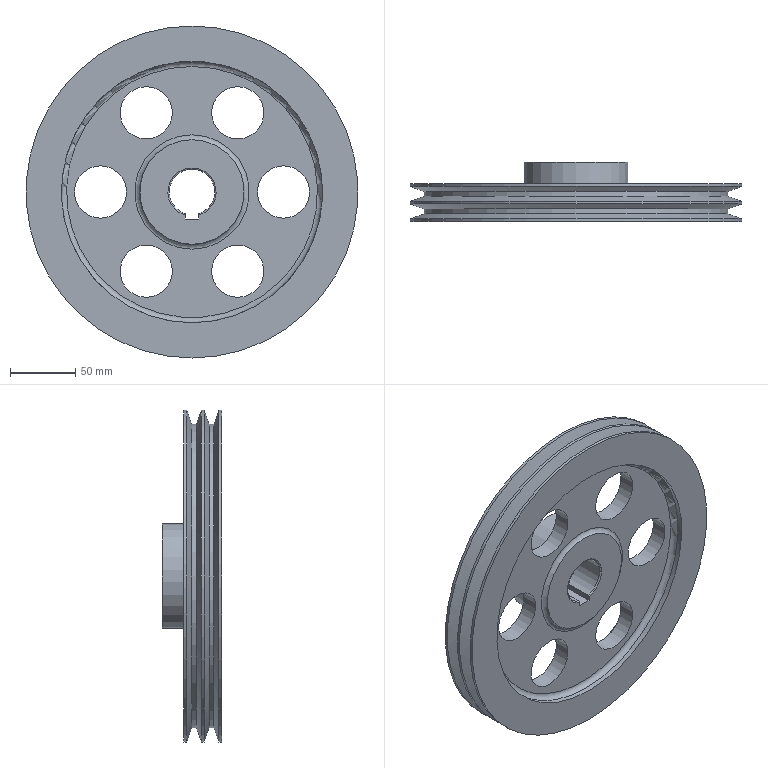Part | NX | features DATUM_CSYS 9, SKETCH 8, EXTRACT_DATUM_AXIS 6, EXTRACT_FACE 6, HOLE PACKAGE 6, SIMPLE HOLE 6, Instance Feature 5, BLEND 2, EXTRUDE 1, Pattern Feature 1, SWP104 1 | 1 solid | 34 faces | box 254 x 45.355 x 254 mm | volume 836856 mm3 | cylinder 15 | plane 9 | torus 6 | cone 4 | commonest cylinder face diameters 40 x6 254 x3 200 x2 232 x2 35 x1 80 x1
STEP:
#1=CARTESIAN_POINT('',(0.,0.,-40.));
#2=VERTEX_POINT('',#1);
#3=CARTESIAN_POINT('',(0.,0.,0.));
#4=DIRECTION('',(0.,-1.,0.));
#5=DIRECTION('',(0.,0.,-1.));
#6=AXIS2_PLACEMENT_3D('',#3,#4,#5);
#7=CIRCLE('',#6,40.);
#8=EDGE_CURVE('',#2,#2,#7,.T.);
#9=ORIENTED_EDGE('',*,*,#8,.T.);
#10=EDGE_LOOP('',(#9));
#11=FACE_BOUND('',#10,.T.);
#12=CARTESIAN_POINT('',(-5.,0.,-17.812));
#13=VERTEX_POINT('',#12);
#14=CARTESIAN_POINT('',(-5.,0.,-20.8));
#15=VERTEX_POINT('',#14);
#16=CARTESIAN_POINT('',(-5.,0.,40.));
#17=DIRECTION('',(0.,0.,-1.));
#18=VECTOR('',#17,1000.);
#19=LINE('',#16,#18);
#20=EDGE_CURVE('',#13,#15,#19,.T.);
#21=ORIENTED_EDGE('',*,*,#20,.F.);
#22=CARTESIAN_POINT('',(5.,0.,-17.812));
#23=VERTEX_POINT('',#22);
#24=CARTESIAN_POINT('',(0.,0.,0.));
#25=DIRECTION('',(0.,1.,0.));
#26=DIRECTION('',(0.,0.,1.));
#27=AXIS2_PLACEMENT_3D('',#24,#25,#26);
#28=CIRCLE('',#27,18.5);
#29=EDGE_CURVE('',#13,#23,#28,.T.);
#30=ORIENTED_EDGE('',*,*,#29,.T.);
#31=CARTESIAN_POINT('',(5.,0.,-20.8));
#32=VERTEX_POINT('',#31);
#33=CARTESIAN_POINT('',(5.,0.,40.));
#34=DIRECTION('',(0.,0.,1.));
#35=VECTOR('',#34,1000.);
#36=LINE('',#33,#35);
#37=EDGE_CURVE('',#32,#23,#36,.T.);
#38=ORIENTED_EDGE('',*,*,#37,.F.);
#39=CARTESIAN_POINT('',(0.,0.,-20.8));
#40=DIRECTION('',(1.,0.,0.));
#41=VECTOR('',#40,1000.);
#42=LINE('',#39,#41);
#43=EDGE_CURVE('',#15,#32,#42,.T.);
#44=ORIENTED_EDGE('',*,*,#43,.F.);
#45=EDGE_LOOP('',(#21,#30,#38,#44));
#46=FACE_BOUND('',#45,.T.);
#47=CARTESIAN_POINT('',(0.,0.,40.));
#48=DIRECTION('',(0.,1.,0.));
#49=DIRECTION('',(0.,0.,1.));
#50=AXIS2_PLACEMENT_3D('',#47,#48,#49);
#51=PLANE('',#50);
#52=ADVANCED_FACE('',(#11,#46),#51,.F.);
#53=CARTESIAN_POINT('',(5.,1.,-16.771));
#54=VERTEX_POINT('',#53);
#55=CARTESIAN_POINT('',(5.,39.,-16.771));
#56=VERTEX_POINT('',#55);
#57=CARTESIAN_POINT('',(5.,0.,-16.771));
#58=DIRECTION('',(0.,-1.,0.));
#59=VECTOR('',#58,1000.);
#60=LINE('',#57,#59);
#61=EDGE_CURVE('',#54,#56,#60,.F.);
#62=ORIENTED_EDGE('',*,*,#61,.F.);
#63=CARTESIAN_POINT('',(-5.,1.,-16.771));
#64=VERTEX_POINT('',#63);
#65=CARTESIAN_POINT('',(0.,1.,0.));
#66=DIRECTION('',(0.,1.,0.));
#67=DIRECTION('',(0.,0.,1.));
#68=AXIS2_PLACEMENT_3D('',#65,#66,#67);
#69=CIRCLE('',#68,17.5);
#70=EDGE_CURVE('',#54,#64,#69,.F.);
#71=ORIENTED_EDGE('',*,*,#70,.T.);
#72=CARTESIAN_POINT('',(-5.,39.,-16.771));
#73=VERTEX_POINT('',#72);
#74=CARTESIAN_POINT('',(-5.,0.,-16.771));
#75=DIRECTION('',(0.,-1.,0.));
#76=VECTOR('',#75,1000.);
#77=LINE('',#74,#76);
#78=EDGE_CURVE('',#73,#64,#77,.T.);
#79=ORIENTED_EDGE('',*,*,#78,.F.);
#80=CARTESIAN_POINT('',(0.,39.,0.));
#81=DIRECTION('',(0.,-1.,0.));
#82=DIRECTION('',(0.,0.,-1.));
#83=AXIS2_PLACEMENT_3D('',#80,#81,#82);
#84=CIRCLE('',#83,17.5);
#85=EDGE_CURVE('',#73,#56,#84,.F.);
#86=ORIENTED_EDGE('',*,*,#85,.T.);
#87=EDGE_LOOP('',(#62,#71,#79,#86));
#88=FACE_BOUND('',#87,.T.);
#89=CARTESIAN_POINT('',(0.,0.,0.));
#90=DIRECTION('',(0.,-1.,0.));
#91=DIRECTION('',(0.,0.,-1.));
#92=AXIS2_PLACEMENT_3D('',#89,#90,#91);
#93=CYLINDRICAL_SURFACE('',#92,17.5);
#94=ADVANCED_FACE('',(#88),#93,.F.);
#95=CARTESIAN_POINT('',(0.,40.,-40.));
#96=VERTEX_POINT('',#95);
#97=CARTESIAN_POINT('',(0.,40.,0.));
#98=DIRECTION('',(0.,-1.,0.));
#99=DIRECTION('',(0.,0.,-1.));
#100=AXIS2_PLACEMENT_3D('',#97,#98,#99);
#101=CIRCLE('',#100,40.);
#102=EDGE_CURVE('',#96,#96,#101,.T.);
#103=ORIENTED_EDGE('',*,*,#102,.F.);
#104=EDGE_LOOP('',(#103));
#105=FACE_BOUND('',#104,.T.);
#106=CARTESIAN_POINT('',(5.,40.,-17.812));
#107=VERTEX_POINT('',#106);
#108=CARTESIAN_POINT('',(5.,40.,-20.8));
#109=VERTEX_POINT('',#108);
#110=CARTESIAN_POINT('',(5.,40.,17.5));
#111=DIRECTION('',(0.,0.,-1.));
#112=VECTOR('',#111,1000.);
#113=LINE('',#110,#112);
#114=EDGE_CURVE('',#107,#109,#113,.T.);
#115=ORIENTED_EDGE('',*,*,#114,.F.);
#116=CARTESIAN_POINT('',(-5.,40.,-17.812));
#117=VERTEX_POINT('',#116);
#118=CARTESIAN_POINT('',(0.,40.,0.));
#119=DIRECTION('',(0.,-1.,0.));
#120=DIRECTION('',(0.,0.,-1.));
#121=AXIS2_PLACEMENT_3D('',#118,#119,#120);
#122=CIRCLE('',#121,18.5);
#123=EDGE_CURVE('',#107,#117,#122,.T.);
#124=ORIENTED_EDGE('',*,*,#123,.T.);
#125=CARTESIAN_POINT('',(-5.,40.,-20.8));
#126=VERTEX_POINT('',#125);
#127=CARTESIAN_POINT('',(-5.,40.,17.5));
#128=DIRECTION('',(0.,0.,1.));
#129=VECTOR('',#128,1000.);
#130=LINE('',#127,#129);
#131=EDGE_CURVE('',#126,#117,#130,.T.);
#132=ORIENTED_EDGE('',*,*,#131,.F.);
#133=CARTESIAN_POINT('',(0.,40.,-20.8));
#134=DIRECTION('',(-1.,0.,0.));
#135=VECTOR('',#134,1000.);
#136=LINE('',#133,#135);
#137=EDGE_CURVE('',#109,#126,#136,.T.);
#138=ORIENTED_EDGE('',*,*,#137,.F.);
#139=EDGE_LOOP('',(#115,#124,#132,#138));
#140=FACE_BOUND('',#139,.T.);
#141=CARTESIAN_POINT('',(0.,40.,17.5));
#142=DIRECTION('',(0.,-1.,0.));
#143=DIRECTION('',(0.,0.,-1.));
#144=AXIS2_PLACEMENT_3D('',#141,#142,#143);
#145=PLANE('',#144);
#146=ADVANCED_FACE('',(#105,#140),#145,.F.);
#147=CARTESIAN_POINT('',(0.,-5.355,-100.));
#148=VERTEX_POINT('',#147);
#149=CARTESIAN_POINT('',(0.,-5.355,0.));
#150=DIRECTION('',(0.,-1.,0.));
#151=DIRECTION('',(0.,0.,-1.));
#152=AXIS2_PLACEMENT_3D('',#149,#150,#151);
#153=CIRCLE('',#152,100.);
#154=EDGE_CURVE('',#148,#148,#153,.T.);
#155=ORIENTED_EDGE('',*,*,#154,.F.);
#156=EDGE_LOOP('',(#155));
#157=FACE_BOUND('',#156,.T.);
#158=CARTESIAN_POINT('',(0.,-5.355,-127.));
#159=VERTEX_POINT('',#158);
#160=CARTESIAN_POINT('',(0.,-5.355,0.));
#161=DIRECTION('',(0.,-1.,0.));
#162=DIRECTION('',(0.,0.,-1.));
#163=AXIS2_PLACEMENT_3D('',#160,#161,#162);
#164=CIRCLE('',#163,127.);
#165=EDGE_CURVE('',#159,#159,#164,.T.);
#166=ORIENTED_EDGE('',*,*,#165,.T.);
#167=EDGE_LOOP('',(#166));
#168=FACE_BOUND('',#167,.T.);
#169=CARTESIAN_POINT('',(0.,-5.355,127.));
#170=DIRECTION('',(0.,1.,0.));
#171=DIRECTION('',(0.,0.,1.));
#172=AXIS2_PLACEMENT_3D('',#169,#170,#171);
#173=PLANE('',#172);
#174=ADVANCED_FACE('',(#157,#168),#173,.F.);
#175=CARTESIAN_POINT('',(0.,-1.294,100.));
#176=VERTEX_POINT('',#175);
#177=CARTESIAN_POINT('',(0.,-1.294,0.));
#178=DIRECTION('',(0.,1.,0.));
#179=DIRECTION('',(0.,0.,1.));
#180=AXIS2_PLACEMENT_3D('',#177,#178,#179);
#181=CIRCLE('',#180,100.);
#182=EDGE_CURVE('',#176,#176,#181,.T.);
#183=ORIENTED_EDGE('',*,*,#182,.T.);
#184=EDGE_LOOP('',(#183));
#185=FACE_BOUND('',#184,.T.);
#186=ORIENTED_EDGE('',*,*,#154,.T.);
#187=EDGE_LOOP('',(#186));
#188=FACE_BOUND('',#187,.T.);
#189=CARTESIAN_POINT('',(0.,0.,0.));
#190=DIRECTION('',(0.,-1.,0.));
#191=DIRECTION('',(0.,0.,-1.));
#192=AXIS2_PLACEMENT_3D('',#189,#190,#191);
#193=CYLINDRICAL_SURFACE('',#192,100.);
#194=ADVANCED_FACE('',(#185,#188),#193,.F.);
#195=CARTESIAN_POINT('',(0.,2.706,96.));
#196=VERTEX_POINT('',#195);
#197=CARTESIAN_POINT('',(0.,2.706,0.));
#198=DIRECTION('',(0.,1.,0.));
#199=DIRECTION('',(0.,0.,1.));
#200=AXIS2_PLACEMENT_3D('',#197,#198,#199);
#201=CIRCLE('',#200,96.);
#202=EDGE_CURVE('',#196,#196,#201,.F.);
#203=ORIENTED_EDGE('',*,*,#202,.T.);
#204=EDGE_LOOP('',(#203));
#205=FACE_BOUND('',#204,.T.);
#206=CARTESIAN_POINT('',(-35.,2.706,80.622));
#207=VERTEX_POINT('',#206);
#208=CARTESIAN_POINT('',(-35.,2.706,60.622));
#209=DIRECTION('',(0.,1.,0.));
#210=DIRECTION('',(0.,0.,1.));
#211=AXIS2_PLACEMENT_3D('',#208,#209,#210);
#212=CIRCLE('',#211,20.);
#213=EDGE_CURVE('',#207,#207,#212,.T.);
#214=ORIENTED_EDGE('',*,*,#213,.T.);
#215=EDGE_LOOP('',(#214));
#216=FACE_BOUND('',#215,.T.);
#217=CARTESIAN_POINT('',(35.,2.706,80.622));
#218=VERTEX_POINT('',#217);
#219=CARTESIAN_POINT('',(35.,2.706,60.622));
#220=DIRECTION('',(0.,1.,0.));
#221=DIRECTION('',(0.,0.,1.));
#222=AXIS2_PLACEMENT_3D('',#219,#220,#221);
#223=CIRCLE('',#222,20.);
#224=EDGE_CURVE('',#218,#218,#223,.T.);
#225=ORIENTED_EDGE('',*,*,#224,.T.);
#226=EDGE_LOOP('',(#225));
#227=FACE_BOUND('',#226,.T.);
#228=CARTESIAN_POINT('',(70.,2.706,20.));
#229=VERTEX_POINT('',#228);
#230=CARTESIAN_POINT('',(70.,2.706,0.));
#231=DIRECTION('',(0.,1.,0.));
#232=DIRECTION('',(0.,0.,1.));
#233=AXIS2_PLACEMENT_3D('',#230,#231,#232);
#234=CIRCLE('',#233,20.);
#235=EDGE_CURVE('',#229,#229,#234,.T.);
#236=ORIENTED_EDGE('',*,*,#235,.T.);
#237=EDGE_LOOP('',(#236));
#238=FACE_BOUND('',#237,.T.);
#239=CARTESIAN_POINT('',(35.,2.706,-40.622));
#240=VERTEX_POINT('',#239);
#241=CARTESIAN_POINT('',(35.,2.706,-60.622));
#242=DIRECTION('',(0.,1.,0.));
#243=DIRECTION('',(0.,0.,1.));
#244=AXIS2_PLACEMENT_3D('',#241,#242,#243);
#245=CIRCLE('',#244,20.);
#246=EDGE_CURVE('',#240,#240,#245,.T.);
#247=ORIENTED_EDGE('',*,*,#246,.T.);
#248=EDGE_LOOP('',(#247));
#249=FACE_BOUND('',#248,.T.);
#250=CARTESIAN_POINT('',(-35.,2.706,-40.622));
#251=VERTEX_POINT('',#250);
#252=CARTESIAN_POINT('',(-35.,2.706,-60.622));
#253=DIRECTION('',(0.,1.,0.));
#254=DIRECTION('',(0.,0.,1.));
#255=AXIS2_PLACEMENT_3D('',#252,#253,#254);
#256=CIRCLE('',#255,20.);
#257=EDGE_CURVE('',#251,#251,#256,.T.);
#258=ORIENTED_EDGE('',*,*,#257,.T.);
#259=EDGE_LOOP('',(#258));
#260=FACE_BOUND('',#259,.T.);
#261=CARTESIAN_POINT('',(-70.,2.706,20.));
#262=VERTEX_POINT('',#261);
#263=CARTESIAN_POINT('',(-70.,2.706,0.));
#264=DIRECTION('',(0.,1.,0.));
#265=DIRECTION('',(0.,0.,1.));
#266=AXIS2_PLACEMENT_3D('',#263,#264,#265);
#267=CIRCLE('',#266,20.);
#268=EDGE_CURVE('',#262,#262,#267,.T.);
#269=ORIENTED_EDGE('',*,*,#268,.T.);
#270=EDGE_LOOP('',(#269));
#271=FACE_BOUND('',#270,.T.);
#272=CARTESIAN_POINT('',(0.,2.706,-43.785));
#273=VERTEX_POINT('',#272);
#274=CARTESIAN_POINT('',(0.,2.706,0.));
#275=DIRECTION('',(0.,-1.,0.));
#276=DIRECTION('',(0.,0.,-1.));
#277=AXIS2_PLACEMENT_3D('',#274,#275,#276);
#278=CIRCLE('',#277,43.785);
#279=EDGE_CURVE('',#273,#273,#278,.T.);
#280=ORIENTED_EDGE('',*,*,#279,.F.);
#281=EDGE_LOOP('',(#280));
#282=FACE_BOUND('',#281,.T.);
#283=CARTESIAN_POINT('',(0.,2.706,100.));
#284=DIRECTION('',(0.,1.,0.));
#285=DIRECTION('',(0.,0.,1.));
#286=AXIS2_PLACEMENT_3D('',#283,#284,#285);
#287=PLANE('',#286);
#288=ADVANCED_FACE('',(#205,#216,#227,#238,#249,#260,#271,#282),#287,.F.);
#289=ORIENTED_EDGE('',*,*,#8,.F.);
#290=EDGE_LOOP('',(#289));
#291=FACE_BOUND('',#290,.T.);
#292=ORIENTED_EDGE('',*,*,#279,.T.);
#293=EDGE_LOOP('',(#292));
#294=FACE_BOUND('',#293,.T.);
#295=CARTESIAN_POINT('',(0.,-1.294,0.));
#296=DIRECTION('',(0.,-1.,0.));
#297=DIRECTION('',(0.,0.,-1.));
#298=AXIS2_PLACEMENT_3D('',#295,#296,#297);
#299=TOROIDAL_SURFACE('',#298,43.785,4.);
#300=ADVANCED_FACE('',(#291,#294),#299,.F.);
#301=CARTESIAN_POINT('',(0.,19.495,-40.));
#302=VERTEX_POINT('',#301);
#303=CARTESIAN_POINT('',(0.,19.495,0.));
#304=DIRECTION('',(0.,-1.,0.));
#305=DIRECTION('',(0.,0.,-1.));
#306=AXIS2_PLACEMENT_3D('',#303,#304,#305);
#307=CIRCLE('',#306,40.);
#308=EDGE_CURVE('',#302,#302,#307,.F.);
#309=ORIENTED_EDGE('',*,*,#308,.T.);
#310=EDGE_LOOP('',(#309));
#311=FACE_BOUND('',#310,.T.);
#312=ORIENTED_EDGE('',*,*,#102,.T.);
#313=EDGE_LOOP('',(#312));
#314=FACE_BOUND('',#313,.T.);
#315=CARTESIAN_POINT('',(0.,0.,0.));
#316=DIRECTION('',(0.,-1.,0.));
#317=DIRECTION('',(0.,0.,-1.));
#318=AXIS2_PLACEMENT_3D('',#315,#316,#317);
#319=CYLINDRICAL_SURFACE('',#318,40.);
#320=ADVANCED_FACE('',(#311,#314),#319,.T.);
#321=CARTESIAN_POINT('',(0.,15.495,-44.));
#322=VERTEX_POINT('',#321);
#323=CARTESIAN_POINT('',(0.,15.495,0.));
#324=DIRECTION('',(0.,-1.,0.));
#325=DIRECTION('',(0.,0.,-1.));
#326=AXIS2_PLACEMENT_3D('',#323,#324,#325);
#327=CIRCLE('',#326,44.);
#328=EDGE_CURVE('',#322,#322,#327,.T.);
#329=ORIENTED_EDGE('',*,*,#328,.T.);
#330=EDGE_LOOP('',(#329));
#331=FACE_BOUND('',#330,.T.);
#332=CARTESIAN_POINT('',(0.,15.495,-96.));
#333=VERTEX_POINT('',#332);
#334=CARTESIAN_POINT('',(0.,15.495,0.));
#335=DIRECTION('',(0.,-1.,0.));
#336=DIRECTION('',(0.,0.,-1.));
#337=AXIS2_PLACEMENT_3D('',#334,#335,#336);
#338=CIRCLE('',#337,96.);
#339=EDGE_CURVE('',#333,#333,#338,.F.);
#340=ORIENTED_EDGE('',*,*,#339,.T.);
#341=EDGE_LOOP('',(#340));
#342=FACE_BOUND('',#341,.T.);
#343=CARTESIAN_POINT('',(-35.,15.495,40.622));
#344=VERTEX_POINT('',#343);
#345=CARTESIAN_POINT('',(-35.,15.495,60.622));
#346=DIRECTION('',(0.,-1.,0.));
#347=DIRECTION('',(0.,0.,-1.));
#348=AXIS2_PLACEMENT_3D('',#345,#346,#347);
#349=CIRCLE('',#348,20.);
#350=EDGE_CURVE('',#344,#344,#349,.T.);
#351=ORIENTED_EDGE('',*,*,#350,.T.);
#352=EDGE_LOOP('',(#351));
#353=FACE_BOUND('',#352,.T.);
#354=CARTESIAN_POINT('',(35.,15.495,40.622));
#355=VERTEX_POINT('',#354);
#356=CARTESIAN_POINT('',(35.,15.495,60.622));
#357=DIRECTION('',(0.,-1.,0.));
#358=DIRECTION('',(0.,0.,-1.));
#359=AXIS2_PLACEMENT_3D('',#356,#357,#358);
#360=CIRCLE('',#359,20.);
#361=EDGE_CURVE('',#355,#355,#360,.T.);
#362=ORIENTED_EDGE('',*,*,#361,.T.);
#363=EDGE_LOOP('',(#362));
#364=FACE_BOUND('',#363,.T.);
#365=CARTESIAN_POINT('',(70.,15.495,-20.));
#366=VERTEX_POINT('',#365);
#367=CARTESIAN_POINT('',(70.,15.495,0.));
#368=DIRECTION('',(0.,-1.,0.));
#369=DIRECTION('',(0.,0.,-1.));
#370=AXIS2_PLACEMENT_3D('',#367,#368,#369);
#371=CIRCLE('',#370,20.);
#372=EDGE_CURVE('',#366,#366,#371,.T.);
#373=ORIENTED_EDGE('',*,*,#372,.T.);
#374=EDGE_LOOP('',(#373));
#375=FACE_BOUND('',#374,.T.);
#376=CARTESIAN_POINT('',(35.,15.495,-80.622));
#377=VERTEX_POINT('',#376);
#378=CARTESIAN_POINT('',(35.,15.495,-60.622));
#379=DIRECTION('',(0.,-1.,0.));
#380=DIRECTION('',(0.,0.,-1.));
#381=AXIS2_PLACEMENT_3D('',#378,#379,#380);
#382=CIRCLE('',#381,20.);
#383=EDGE_CURVE('',#377,#377,#382,.T.);
#384=ORIENTED_EDGE('',*,*,#383,.T.);
#385=EDGE_LOOP('',(#384));
#386=FACE_BOUND('',#385,.T.);
#387=CARTESIAN_POINT('',(-35.,15.495,-80.622));
#388=VERTEX_POINT('',#387);
#389=CARTESIAN_POINT('',(-35.,15.495,-60.622));
#390=DIRECTION('',(0.,-1.,0.));
#391=DIRECTION('',(0.,0.,-1.));
#392=AXIS2_PLACEMENT_3D('',#389,#390,#391);
#393=CIRCLE('',#392,20.);
#394=EDGE_CURVE('',#388,#388,#393,.T.);
#395=ORIENTED_EDGE('',*,*,#394,.T.);
#396=EDGE_LOOP('',(#395));
#397=FACE_BOUND('',#396,.T.);
#398=CARTESIAN_POINT('',(-70.,15.495,-20.));
#399=VERTEX_POINT('',#398);
#400=CARTESIAN_POINT('',(-70.,15.495,0.));
#401=DIRECTION('',(0.,-1.,0.));
#402=DIRECTION('',(0.,0.,-1.));
#403=AXIS2_PLACEMENT_3D('',#400,#401,#402);
#404=CIRCLE('',#403,20.);
#405=EDGE_CURVE('',#399,#399,#404,.T.);
#406=ORIENTED_EDGE('',*,*,#405,.T.);
#407=EDGE_LOOP('',(#406));
#408=FACE_BOUND('',#407,.T.);
#409=CARTESIAN_POINT('',(0.,15.495,40.));
#410=DIRECTION('',(0.,-1.,0.));
#411=DIRECTION('',(0.,0.,-1.));
#412=AXIS2_PLACEMENT_3D('',#409,#410,#411);
#413=PLANE('',#412);
#414=ADVANCED_FACE('',(#331,#342,#353,#364,#375,#386,#397,#408),#413,.F.);
#415=CARTESIAN_POINT('',(0.,19.495,-100.));
#416=VERTEX_POINT('',#415);
#417=CARTESIAN_POINT('',(0.,19.495,0.));
#418=DIRECTION('',(0.,-1.,0.));
#419=DIRECTION('',(0.,0.,-1.));
#420=AXIS2_PLACEMENT_3D('',#417,#418,#419);
#421=CIRCLE('',#420,100.);
#422=EDGE_CURVE('',#416,#416,#421,.T.);
#423=ORIENTED_EDGE('',*,*,#422,.T.);
#424=EDGE_LOOP('',(#423));
#425=FACE_BOUND('',#424,.T.);
#426=CARTESIAN_POINT('',(0.,23.495,-100.));
#427=VERTEX_POINT('',#426);
#428=CARTESIAN_POINT('',(0.,23.495,0.));
#429=DIRECTION('',(0.,-1.,0.));
#430=DIRECTION('',(0.,0.,-1.));
#431=AXIS2_PLACEMENT_3D('',#428,#429,#430);
#432=CIRCLE('',#431,100.);
#433=EDGE_CURVE('',#427,#427,#432,.T.);
#434=ORIENTED_EDGE('',*,*,#433,.F.);
#435=EDGE_LOOP('',(#434));
#436=FACE_BOUND('',#435,.T.);
#437=CARTESIAN_POINT('',(0.,0.,0.));
#438=DIRECTION('',(0.,-1.,0.));
#439=DIRECTION('',(0.,0.,-1.));
#440=AXIS2_PLACEMENT_3D('',#437,#438,#439);
#441=CYLINDRICAL_SURFACE('',#440,100.);
#442=ADVANCED_FACE('',(#425,#436),#441,.F.);
#443=CARTESIAN_POINT('',(0.,23.495,-127.));
#444=VERTEX_POINT('',#443);
#445=CARTESIAN_POINT('',(0.,23.495,0.));
#446=DIRECTION('',(0.,-1.,0.));
#447=DIRECTION('',(0.,0.,-1.));
#448=AXIS2_PLACEMENT_3D('',#445,#446,#447);
#449=CIRCLE('',#448,127.);
#450=EDGE_CURVE('',#444,#444,#449,.T.);
#451=ORIENTED_EDGE('',*,*,#450,.F.);
#452=EDGE_LOOP('',(#451));
#453=FACE_BOUND('',#452,.T.);
#454=ORIENTED_EDGE('',*,*,#433,.T.);
#455=EDGE_LOOP('',(#454));
#456=FACE_BOUND('',#455,.T.);
#457=CARTESIAN_POINT('',(0.,23.495,100.));
#458=DIRECTION('',(0.,-1.,0.));
#459=DIRECTION('',(0.,0.,-1.));
#460=AXIS2_PLACEMENT_3D('',#457,#458,#459);
#461=PLANE('',#460);
#462=ADVANCED_FACE('',(#453,#456),#461,.F.);
#463=CARTESIAN_POINT('',(0.,21.395,-127.));
#464=VERTEX_POINT('',#463);
#465=CARTESIAN_POINT('',(0.,21.395,0.));
#466=DIRECTION('',(0.,-1.,0.));
#467=DIRECTION('',(0.,0.,-1.));
#468=AXIS2_PLACEMENT_3D('',#465,#466,#467);
#469=CIRCLE('',#468,127.);
#470=EDGE_CURVE('',#464,#464,#469,.T.);
#471=ORIENTED_EDGE('',*,*,#470,.F.);
#472=EDGE_LOOP('',(#471));
#473=FACE_BOUND('',#472,.T.);
#474=ORIENTED_EDGE('',*,*,#450,.T.);
#475=EDGE_LOOP('',(#474));
#476=FACE_BOUND('',#475,.T.);
#477=CARTESIAN_POINT('',(0.,0.,0.));
#478=DIRECTION('',(0.,-1.,0.));
#479=DIRECTION('',(0.,0.,-1.));
#480=AXIS2_PLACEMENT_3D('',#477,#478,#479);
#481=CYLINDRICAL_SURFACE('',#480,127.);
#482=ADVANCED_FACE('',(#473,#476),#481,.T.);
#483=CARTESIAN_POINT('',(0.,17.608,-116.));
#484=VERTEX_POINT('',#483);
#485=CARTESIAN_POINT('',(0.,17.608,0.));
#486=DIRECTION('',(0.,-1.,0.));
#487=DIRECTION('',(0.,0.,-1.));
#488=AXIS2_PLACEMENT_3D('',#485,#486,#487);
#489=CIRCLE('',#488,116.);
#490=EDGE_CURVE('',#484,#484,#489,.T.);
#491=ORIENTED_EDGE('',*,*,#490,.F.);
#492=EDGE_LOOP('',(#491));
#493=FACE_BOUND('',#492,.T.);
#494=ORIENTED_EDGE('',*,*,#470,.T.);
#495=EDGE_LOOP('',(#494));
#496=FACE_BOUND('',#495,.T.);
#497=CARTESIAN_POINT('',(0.,21.395,0.));
#498=DIRECTION('',(0.,1.,0.));
#499=DIRECTION('',(0.,0.,1.));
#500=AXIS2_PLACEMENT_3D('',#497,#498,#499);
#501=CONICAL_SURFACE('',#500,127.,1.239);
#502=ADVANCED_FACE('',(#493,#496),#501,.T.);
#503=CARTESIAN_POINT('',(0.,13.908,-116.));
#504=VERTEX_POINT('',#503);
#505=CARTESIAN_POINT('',(0.,13.908,0.));
#506=DIRECTION('',(0.,-1.,0.));
#507=DIRECTION('',(0.,0.,-1.));
#508=AXIS2_PLACEMENT_3D('',#505,#506,#507);
#509=CIRCLE('',#508,116.);
#510=EDGE_CURVE('',#504,#504,#509,.T.);
#511=ORIENTED_EDGE('',*,*,#510,.F.);
#512=EDGE_LOOP('',(#511));
#513=FACE_BOUND('',#512,.T.);
#514=ORIENTED_EDGE('',*,*,#490,.T.);
#515=EDGE_LOOP('',(#514));
#516=FACE_BOUND('',#515,.T.);
#517=CARTESIAN_POINT('',(0.,0.,0.));
#518=DIRECTION('',(0.,-1.,0.));
#519=DIRECTION('',(0.,0.,-1.));
#520=AXIS2_PLACEMENT_3D('',#517,#518,#519);
#521=CYLINDRICAL_SURFACE('',#520,116.);
#522=ADVANCED_FACE('',(#513,#516),#521,.T.);
#523=CARTESIAN_POINT('',(0.,10.12,-127.));
#524=VERTEX_POINT('',#523);
#525=CARTESIAN_POINT('',(0.,10.12,0.));
#526=DIRECTION('',(0.,-1.,0.));
#527=DIRECTION('',(0.,0.,-1.));
#528=AXIS2_PLACEMENT_3D('',#525,#526,#527);
#529=CIRCLE('',#528,127.);
#530=EDGE_CURVE('',#524,#524,#529,.T.);
#531=ORIENTED_EDGE('',*,*,#530,.F.);
#532=EDGE_LOOP('',(#531));
#533=FACE_BOUND('',#532,.T.);
#534=ORIENTED_EDGE('',*,*,#510,.T.);
#535=EDGE_LOOP('',(#534));
#536=FACE_BOUND('',#535,.T.);
#537=CARTESIAN_POINT('',(0.,13.908,0.));
#538=DIRECTION('',(0.,-1.,0.));
#539=DIRECTION('',(0.,0.,-1.));
#540=AXIS2_PLACEMENT_3D('',#537,#538,#539);
#541=CONICAL_SURFACE('',#540,116.,1.239);
#542=ADVANCED_FACE('',(#533,#536),#541,.T.);
#543=CARTESIAN_POINT('',(0.,8.02,-127.));
#544=VERTEX_POINT('',#543);
#545=CARTESIAN_POINT('',(0.,8.02,0.));
#546=DIRECTION('',(0.,-1.,0.));
#547=DIRECTION('',(0.,0.,-1.));
#548=AXIS2_PLACEMENT_3D('',#545,#546,#547);
#549=CIRCLE('',#548,127.);
#550=EDGE_CURVE('',#544,#544,#549,.T.);
#551=ORIENTED_EDGE('',*,*,#550,.F.);
#552=EDGE_LOOP('',(#551));
#553=FACE_BOUND('',#552,.T.);
#554=ORIENTED_EDGE('',*,*,#530,.T.);
#555=EDGE_LOOP('',(#554));
#556=FACE_BOUND('',#555,.T.);
#557=CARTESIAN_POINT('',(0.,0.,0.));
#558=DIRECTION('',(0.,-1.,0.));
#559=DIRECTION('',(0.,0.,-1.));
#560=AXIS2_PLACEMENT_3D('',#557,#558,#559);
#561=CYLINDRICAL_SURFACE('',#560,127.);
#562=ADVANCED_FACE('',(#553,#556),#561,.T.);
#563=CARTESIAN_POINT('',(0.,4.233,-116.));
#564=VERTEX_POINT('',#563);
#565=CARTESIAN_POINT('',(0.,4.233,0.));
#566=DIRECTION('',(0.,-1.,0.));
#567=DIRECTION('',(0.,0.,-1.));
#568=AXIS2_PLACEMENT_3D('',#565,#566,#567);
#569=CIRCLE('',#568,116.);
#570=EDGE_CURVE('',#564,#564,#569,.T.);
#571=ORIENTED_EDGE('',*,*,#570,.F.);
#572=EDGE_LOOP('',(#571));
#573=FACE_BOUND('',#572,.T.);
#574=ORIENTED_EDGE('',*,*,#550,.T.);
#575=EDGE_LOOP('',(#574));
#576=FACE_BOUND('',#575,.T.);
#577=CARTESIAN_POINT('',(0.,8.02,0.));
#578=DIRECTION('',(0.,1.,0.));
#579=DIRECTION('',(0.,0.,1.));
#580=AXIS2_PLACEMENT_3D('',#577,#578,#579);
#581=CONICAL_SURFACE('',#580,127.,1.239);
#582=ADVANCED_FACE('',(#573,#576),#581,.T.);
#583=CARTESIAN_POINT('',(0.,0.5326,-116.));
#584=VERTEX_POINT('',#583);
#585=CARTESIAN_POINT('',(0.,0.5326,0.));
#586=DIRECTION('',(0.,-1.,0.));
#587=DIRECTION('',(0.,0.,-1.));
#588=AXIS2_PLACEMENT_3D('',#585,#586,#587);
#589=CIRCLE('',#588,116.);
#590=EDGE_CURVE('',#584,#584,#589,.T.);
#591=ORIENTED_EDGE('',*,*,#590,.F.);
#592=EDGE_LOOP('',(#591));
#593=FACE_BOUND('',#592,.T.);
#594=ORIENTED_EDGE('',*,*,#570,.T.);
#595=EDGE_LOOP('',(#594));
#596=FACE_BOUND('',#595,.T.);
#597=CARTESIAN_POINT('',(0.,0.,0.));
#598=DIRECTION('',(0.,-1.,0.));
#599=DIRECTION('',(0.,0.,-1.));
#600=AXIS2_PLACEMENT_3D('',#597,#598,#599);
#601=CYLINDRICAL_SURFACE('',#600,116.);
#602=ADVANCED_FACE('',(#593,#596),#601,.T.);
#603=CARTESIAN_POINT('',(0.,-3.255,-127.));
#604=VERTEX_POINT('',#603);
#605=CARTESIAN_POINT('',(0.,-3.255,0.));
#606=DIRECTION('',(0.,-1.,0.));
#607=DIRECTION('',(0.,0.,-1.));
#608=AXIS2_PLACEMENT_3D('',#605,#606,#607);
#609=CIRCLE('',#608,127.);
#610=EDGE_CURVE('',#604,#604,#609,.T.);
#611=ORIENTED_EDGE('',*,*,#610,.F.);
#612=EDGE_LOOP('',(#611));
#613=FACE_BOUND('',#612,.T.);
#614=ORIENTED_EDGE('',*,*,#590,.T.);
#615=EDGE_LOOP('',(#614));
#616=FACE_BOUND('',#615,.T.);
#617=CARTESIAN_POINT('',(0.,0.5326,0.));
#618=DIRECTION('',(0.,-1.,0.));
#619=DIRECTION('',(0.,0.,-1.));
#620=AXIS2_PLACEMENT_3D('',#617,#618,#619);
#621=CONICAL_SURFACE('',#620,116.,1.239);
#622=ADVANCED_FACE('',(#613,#616),#621,.T.);
#623=ORIENTED_EDGE('',*,*,#165,.F.);
#624=EDGE_LOOP('',(#623));
#625=FACE_BOUND('',#624,.T.);
#626=ORIENTED_EDGE('',*,*,#610,.T.);
#627=EDGE_LOOP('',(#626));
#628=FACE_BOUND('',#627,.T.);
#629=CARTESIAN_POINT('',(0.,0.,0.));
#630=DIRECTION('',(0.,-1.,0.));
#631=DIRECTION('',(0.,0.,-1.));
#632=AXIS2_PLACEMENT_3D('',#629,#630,#631);
#633=CYLINDRICAL_SURFACE('',#632,127.);
#634=ADVANCED_FACE('',(#625,#628),#633,.T.);
#635=ORIENTED_EDGE('',*,*,#405,.F.);
#636=EDGE_LOOP('',(#635));
#637=FACE_BOUND('',#636,.T.);
#638=ORIENTED_EDGE('',*,*,#268,.F.);
#639=EDGE_LOOP('',(#638));
#640=FACE_BOUND('',#639,.T.);
#641=CARTESIAN_POINT('',(-70.,15.495,0.));
#642=DIRECTION('',(0.,-1.,0.));
#643=DIRECTION('',(0.,0.,-1.));
#644=AXIS2_PLACEMENT_3D('',#641,#642,#643);
#645=CYLINDRICAL_SURFACE('',#644,20.);
#646=ADVANCED_FACE('',(#637,#640),#645,.F.);
#647=ORIENTED_EDGE('',*,*,#394,.F.);
#648=EDGE_LOOP('',(#647));
#649=FACE_BOUND('',#648,.T.);
#650=ORIENTED_EDGE('',*,*,#257,.F.);
#651=EDGE_LOOP('',(#650));
#652=FACE_BOUND('',#651,.T.);
#653=CARTESIAN_POINT('',(-35.,15.495,-60.622));
#654=DIRECTION('',(0.,-1.,0.));
#655=DIRECTION('',(0.,0.,-1.));
#656=AXIS2_PLACEMENT_3D('',#653,#654,#655);
#657=CYLINDRICAL_SURFACE('',#656,20.);
#658=ADVANCED_FACE('',(#649,#652),#657,.F.);
#659=ORIENTED_EDGE('',*,*,#383,.F.);
#660=EDGE_LOOP('',(#659));
#661=FACE_BOUND('',#660,.T.);
#662=ORIENTED_EDGE('',*,*,#246,.F.);
#663=EDGE_LOOP('',(#662));
#664=FACE_BOUND('',#663,.T.);
#665=CARTESIAN_POINT('',(35.,15.495,-60.622));
#666=DIRECTION('',(0.,-1.,0.));
#667=DIRECTION('',(0.,0.,-1.));
#668=AXIS2_PLACEMENT_3D('',#665,#666,#667);
#669=CYLINDRICAL_SURFACE('',#668,20.);
#670=ADVANCED_FACE('',(#661,#664),#669,.F.);
#671=ORIENTED_EDGE('',*,*,#372,.F.);
#672=EDGE_LOOP('',(#671));
#673=FACE_BOUND('',#672,.T.);
#674=ORIENTED_EDGE('',*,*,#235,.F.);
#675=EDGE_LOOP('',(#674));
#676=FACE_BOUND('',#675,.T.);
#677=CARTESIAN_POINT('',(70.,15.495,0.));
#678=DIRECTION('',(0.,-1.,0.));
#679=DIRECTION('',(0.,0.,-1.));
#680=AXIS2_PLACEMENT_3D('',#677,#678,#679);
#681=CYLINDRICAL_SURFACE('',#680,20.);
#682=ADVANCED_FACE('',(#673,#676),#681,.F.);
#683=ORIENTED_EDGE('',*,*,#361,.F.);
#684=EDGE_LOOP('',(#683));
#685=FACE_BOUND('',#684,.T.);
#686=ORIENTED_EDGE('',*,*,#224,.F.);
#687=EDGE_LOOP('',(#686));
#688=FACE_BOUND('',#687,.T.);
#689=CARTESIAN_POINT('',(35.,15.495,60.622));
#690=DIRECTION('',(0.,-1.,0.));
#691=DIRECTION('',(0.,0.,-1.));
#692=AXIS2_PLACEMENT_3D('',#689,#690,#691);
#693=CYLINDRICAL_SURFACE('',#692,20.);
#694=ADVANCED_FACE('',(#685,#688),#693,.F.);
#695=ORIENTED_EDGE('',*,*,#350,.F.);
#696=EDGE_LOOP('',(#695));
#697=FACE_BOUND('',#696,.T.);
#698=ORIENTED_EDGE('',*,*,#213,.F.);
#699=EDGE_LOOP('',(#698));
#700=FACE_BOUND('',#699,.T.);
#701=CARTESIAN_POINT('',(-35.,15.495,60.622));
#702=DIRECTION('',(0.,-1.,0.));
#703=DIRECTION('',(0.,0.,-1.));
#704=AXIS2_PLACEMENT_3D('',#701,#702,#703);
#705=CYLINDRICAL_SURFACE('',#704,20.);
#706=ADVANCED_FACE('',(#697,#700),#705,.F.);
#707=ORIENTED_EDGE('',*,*,#78,.T.);
#708=CARTESIAN_POINT('',(-5.,1.,-16.771));
#709=CARTESIAN_POINT('',(-5.,0.4608,-16.771));
#710=CARTESIAN_POINT('',(-5.,0.,-17.273));
#711=CARTESIAN_POINT('',(-5.,0.,-17.812));
#712=B_SPLINE_CURVE_WITH_KNOTS('',3,(#708,#709,#710,#711),.UNSPECIFIED.,.F.,.F.,(4,4),(0.,0.001594),.UNSPECIFIED.);
#713=EDGE_CURVE('',#64,#13,#712,.T.);
#714=ORIENTED_EDGE('',*,*,#713,.T.);
#715=ORIENTED_EDGE('',*,*,#20,.T.);
#716=CARTESIAN_POINT('',(-5.,-69.,-20.8));
#717=DIRECTION('',(0.,1.,0.));
#718=VECTOR('',#717,1000.);
#719=LINE('',#716,#718);
#720=EDGE_CURVE('',#126,#15,#719,.F.);
#721=ORIENTED_EDGE('',*,*,#720,.F.);
#722=ORIENTED_EDGE('',*,*,#131,.T.);
#723=CARTESIAN_POINT('',(-5.,40.,-17.812));
#724=CARTESIAN_POINT('',(-5.,40.,-17.273));
#725=CARTESIAN_POINT('',(-5.,39.54,-16.771));
#726=CARTESIAN_POINT('',(-5.,39.,-16.771));
#727=B_SPLINE_CURVE_WITH_KNOTS('',3,(#723,#724,#725,#726),.UNSPECIFIED.,.F.,.F.,(4,4),(0.,0.001594),.UNSPECIFIED.);
#728=EDGE_CURVE('',#117,#73,#727,.T.);
#729=ORIENTED_EDGE('',*,*,#728,.T.);
#730=EDGE_LOOP('',(#707,#714,#715,#721,#722,#729));
#731=FACE_BOUND('',#730,.T.);
#732=CARTESIAN_POINT('',(-5.,-69.,-5.3));
#733=DIRECTION('',(1.,0.,0.));
#734=DIRECTION('',(0.,0.,-1.));
#735=AXIS2_PLACEMENT_3D('',#732,#733,#734);
#736=PLANE('',#735);
#737=ADVANCED_FACE('',(#731),#736,.T.);
#738=ORIENTED_EDGE('',*,*,#43,.T.);
#739=CARTESIAN_POINT('',(5.,-69.,-20.8));
#740=DIRECTION('',(0.,1.,0.));
#741=VECTOR('',#740,1000.);
#742=LINE('',#739,#741);
#743=EDGE_CURVE('',#109,#32,#742,.F.);
#744=ORIENTED_EDGE('',*,*,#743,.F.);
#745=ORIENTED_EDGE('',*,*,#137,.T.);
#746=ORIENTED_EDGE('',*,*,#720,.T.);
#747=EDGE_LOOP('',(#738,#744,#745,#746));
#748=FACE_BOUND('',#747,.T.);
#749=CARTESIAN_POINT('',(-5.,-69.,-20.8));
#750=DIRECTION('',(0.,0.,1.));
#751=DIRECTION('',(1.,0.,0.));
#752=AXIS2_PLACEMENT_3D('',#749,#750,#751);
#753=PLANE('',#752);
#754=ADVANCED_FACE('',(#748),#753,.T.);
#755=ORIENTED_EDGE('',*,*,#37,.T.);
#756=CARTESIAN_POINT('',(5.,0.,-17.812));
#757=CARTESIAN_POINT('',(5.,0.,-17.273));
#758=CARTESIAN_POINT('',(5.,0.4604,-16.771));
#759=CARTESIAN_POINT('',(5.,1.,-16.771));
#760=B_SPLINE_CURVE_WITH_KNOTS('',3,(#756,#757,#758,#759),.UNSPECIFIED.,.F.,.F.,(4,4),(0.,0.001594),.UNSPECIFIED.);
#761=EDGE_CURVE('',#23,#54,#760,.T.);
#762=ORIENTED_EDGE('',*,*,#761,.T.);
#763=ORIENTED_EDGE('',*,*,#61,.T.);
#764=CARTESIAN_POINT('',(5.,39.,-16.771));
#765=CARTESIAN_POINT('',(5.,39.539,-16.771));
#766=CARTESIAN_POINT('',(5.,40.,-17.273));
#767=CARTESIAN_POINT('',(5.,40.,-17.812));
#768=B_SPLINE_CURVE_WITH_KNOTS('',3,(#764,#765,#766,#767),.UNSPECIFIED.,.F.,.F.,(4,4),(0.,0.001594),.UNSPECIFIED.);
#769=EDGE_CURVE('',#56,#107,#768,.T.);
#770=ORIENTED_EDGE('',*,*,#769,.T.);
#771=ORIENTED_EDGE('',*,*,#114,.T.);
#772=ORIENTED_EDGE('',*,*,#743,.T.);
#773=EDGE_LOOP('',(#755,#762,#763,#770,#771,#772));
#774=FACE_BOUND('',#773,.T.);
#775=CARTESIAN_POINT('',(5.,-69.,-20.8));
#776=DIRECTION('',(-1.,0.,0.));
#777=DIRECTION('',(0.,0.,1.));
#778=AXIS2_PLACEMENT_3D('',#775,#776,#777);
#779=PLANE('',#778);
#780=ADVANCED_FACE('',(#774),#779,.T.);
#781=ORIENTED_EDGE('',*,*,#182,.F.);
#782=EDGE_LOOP('',(#781));
#783=FACE_BOUND('',#782,.T.);
#784=ORIENTED_EDGE('',*,*,#202,.F.);
#785=EDGE_LOOP('',(#784));
#786=FACE_BOUND('',#785,.T.);
#787=CARTESIAN_POINT('',(0.,-1.294,0.));
#788=DIRECTION('',(0.,1.,0.));
#789=DIRECTION('',(0.,0.,1.));
#790=AXIS2_PLACEMENT_3D('',#787,#788,#789);
#791=TOROIDAL_SURFACE('',#790,96.,4.);
#792=ADVANCED_FACE('',(#783,#786),#791,.F.);
#793=ORIENTED_EDGE('',*,*,#308,.F.);
#794=EDGE_LOOP('',(#793));
#795=FACE_BOUND('',#794,.T.);
#796=ORIENTED_EDGE('',*,*,#328,.F.);
#797=EDGE_LOOP('',(#796));
#798=FACE_BOUND('',#797,.T.);
#799=CARTESIAN_POINT('',(0.,19.495,0.));
#800=DIRECTION('',(0.,-1.,0.));
#801=DIRECTION('',(0.,0.,-1.));
#802=AXIS2_PLACEMENT_3D('',#799,#800,#801);
#803=TOROIDAL_SURFACE('',#802,44.,4.);
#804=ADVANCED_FACE('',(#795,#798),#803,.F.);
#805=ORIENTED_EDGE('',*,*,#339,.F.);
#806=EDGE_LOOP('',(#805));
#807=FACE_BOUND('',#806,.T.);
#808=ORIENTED_EDGE('',*,*,#422,.F.);
#809=EDGE_LOOP('',(#808));
#810=FACE_BOUND('',#809,.T.);
#811=CARTESIAN_POINT('',(0.,19.495,0.));
#812=DIRECTION('',(0.,-1.,0.));
#813=DIRECTION('',(0.,0.,-1.));
#814=AXIS2_PLACEMENT_3D('',#811,#812,#813);
#815=TOROIDAL_SURFACE('',#814,96.,4.);
#816=ADVANCED_FACE('',(#807,#810),#815,.F.);
#817=ORIENTED_EDGE('',*,*,#761,.F.);
#818=ORIENTED_EDGE('',*,*,#29,.F.);
#819=ORIENTED_EDGE('',*,*,#713,.F.);
#820=ORIENTED_EDGE('',*,*,#70,.F.);
#821=EDGE_LOOP('',(#817,#818,#819,#820));
#822=FACE_BOUND('',#821,.T.);
#823=CARTESIAN_POINT('',(0.,1.,0.));
#824=DIRECTION('',(0.,1.,0.));
#825=DIRECTION('',(0.,0.,1.));
#826=AXIS2_PLACEMENT_3D('',#823,#824,#825);
#827=TOROIDAL_SURFACE('',#826,18.5,1.);
#828=ADVANCED_FACE('',(#822),#827,.T.);
#829=ORIENTED_EDGE('',*,*,#769,.F.);
#830=ORIENTED_EDGE('',*,*,#85,.F.);
#831=ORIENTED_EDGE('',*,*,#728,.F.);
#832=ORIENTED_EDGE('',*,*,#123,.F.);
#833=EDGE_LOOP('',(#829,#830,#831,#832));
#834=FACE_BOUND('',#833,.T.);
#835=CARTESIAN_POINT('',(0.,39.,0.));
#836=DIRECTION('',(0.,-1.,0.));
#837=DIRECTION('',(0.,0.,-1.));
#838=AXIS2_PLACEMENT_3D('',#835,#836,#837);
#839=TOROIDAL_SURFACE('',#838,18.5,1.);
#840=ADVANCED_FACE('',(#834),#839,.T.);
#841=CLOSED_SHELL('',(#52,#94,#146,#174,#194,#288,#300,#320,#414,#442,#462,#482,#502,#522,#542,#562,#582,#602,#622,#634,#646,#658,#670,#682,#694,#706,#737,#754,#780,#792,#804,#816,#828,#840));
#842=MANIFOLD_SOLID_BREP('',#841);
#843=(LENGTH_UNIT()NAMED_UNIT(*)SI_UNIT(.MILLI.,.METRE.));
#844=UNCERTAINTY_MEASURE_WITH_UNIT(LENGTH_MEASURE(0.0508),#843,'','');
#845=(NAMED_UNIT(*)PLANE_ANGLE_UNIT()SI_UNIT($,.RADIAN.));
#846=(NAMED_UNIT(*)SI_UNIT($,.STERADIAN.)SOLID_ANGLE_UNIT());
#847=(GEOMETRIC_REPRESENTATION_CONTEXT(3)GLOBAL_UNCERTAINTY_ASSIGNED_CONTEXT((#844))GLOBAL_UNIT_ASSIGNED_CONTEXT((#843,#845,#846))REPRESENTATION_CONTEXT('',''));
#848=ADVANCED_BREP_SHAPE_REPRESENTATION('',(#842),#847);